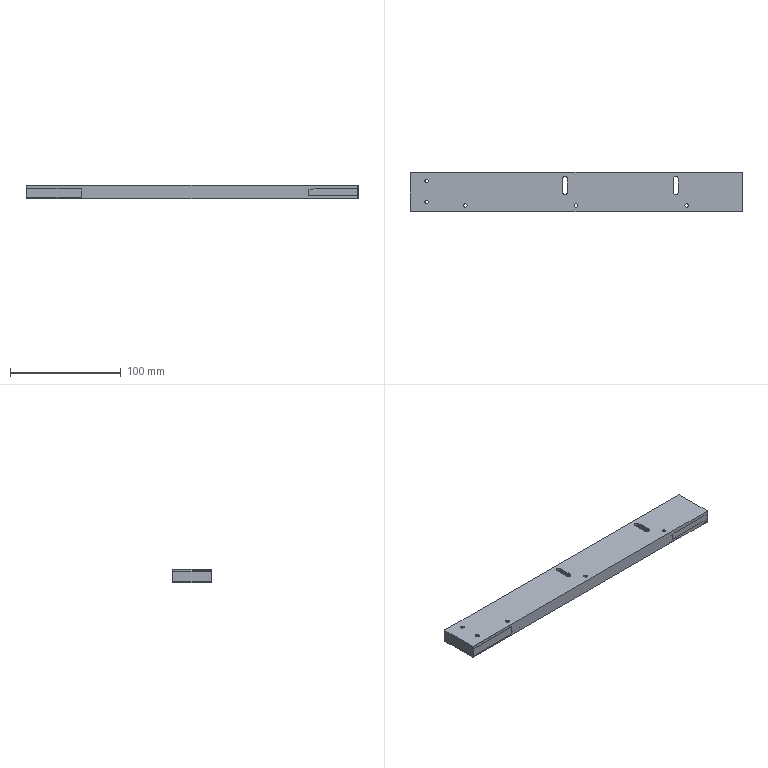Part | 2 solids | 62 faces | box 300 x 36 x 12 mm | volume 225326 mm3 | plane 43 | cylinder 19 | commonest cylinder face diameters 3.242 x10 4.5 x8 2 x1